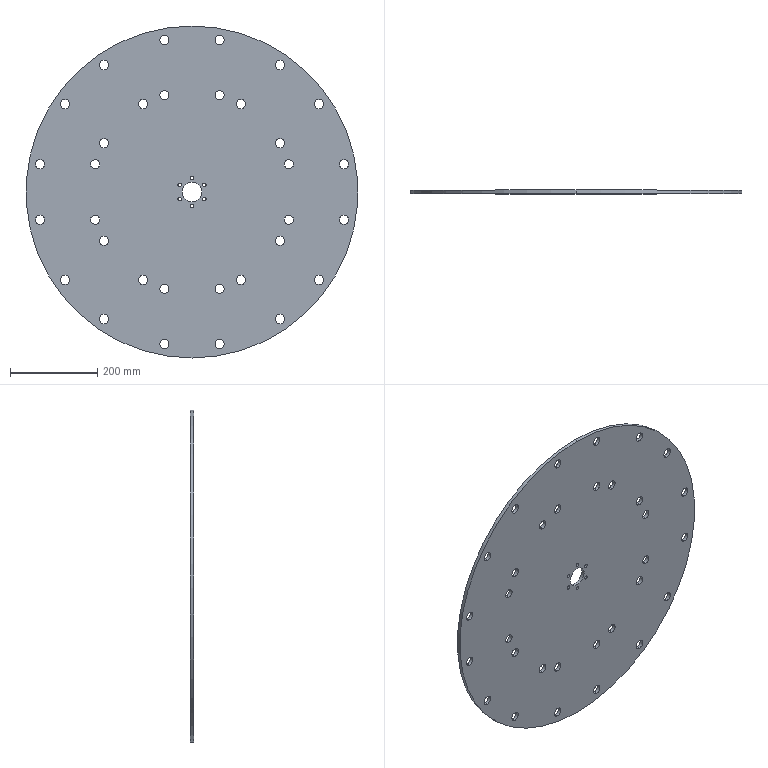Part | 1 solid | 253 faces | box 760 x 8 x 760 mm | volume 3525186 mm3 | spline 115 | cylinder 80 | plane 58 | commonest cylinder face diameters 21 x64 8 x12 45.2 x2 760 x2